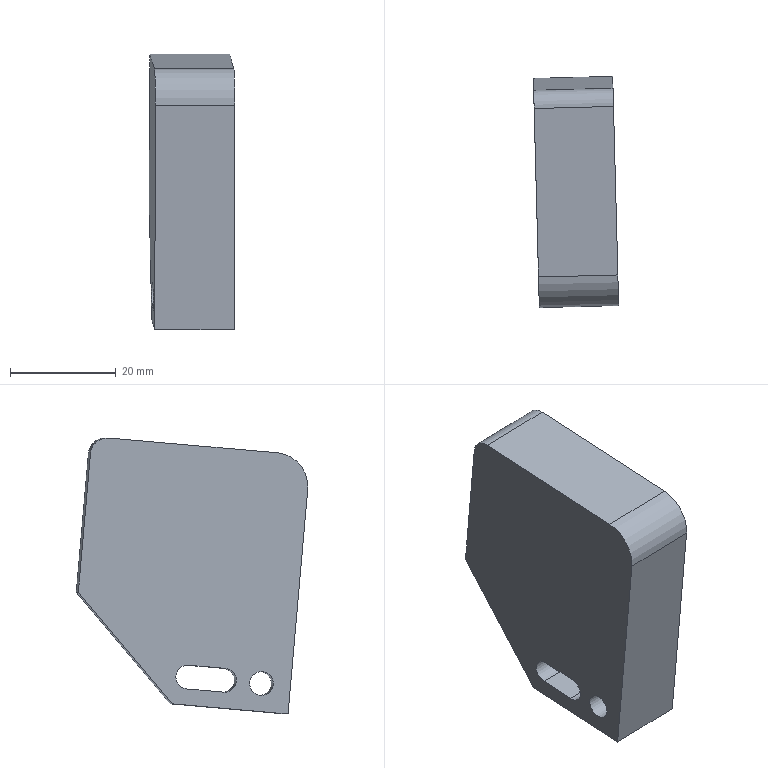Part | STEP file | 1_id1298_x_t | 1 solid | 14 faces | box 16.123 x 43.759 x 52.166 mm | volume 26539 mm3 | plane 9 | cylinder 5 | commonest cylinder face diameters 4.5 x3 6.35 x1 12.7 x1
STEP:
#1=CARTESIAN_POINT('',(0.,0.,0.));
#2=DIRECTION('',(0.,0.,1.));
#3=DIRECTION('',(1.,0.,0.));
#4=AXIS2_PLACEMENT_3D('',#1,#2,#3);
#5=CARTESIAN_POINT('',(981.211,308.005,19.618));
#6=VERTEX_POINT('',#5);
#7=CARTESIAN_POINT('',(966.216,307.615,19.618));
#8=VERTEX_POINT('',#7);
#9=CARTESIAN_POINT('',(981.211,308.005,19.618));
#10=DIRECTION('',(-0.9997,-0.02601,0.));
#11=VECTOR('',#10,1.);
#12=LINE('',#9,#11);
#13=CARTESIAN_POINT('',(981.114,311.721,-22.87));
#14=DIRECTION('',(0.02591,-0.9959,-0.08716));
#15=DIRECTION('',(0.05454,-0.08565,0.9948));
#16=AXIS2_PLACEMENT_3D('',#13,#14,#15);
#17=PLANE('',#16);
#18=CARTESIAN_POINT('',(42.592,2.23));
#19=DIRECTION('',(-0.0523,0.9986));
#20=VECTOR('',#19,1.);
#21=LINE('',#18,#20);
#22=(GEOMETRIC_REPRESENTATION_CONTEXT(2)PARAMETRIC_REPRESENTATION_CONTEXT()REPRESENTATION_CONTEXT('',''));
#23=DEFINITIONAL_REPRESENTATION('',(#21),#22);
#24=PCURVE('',#17,#23);
#25=CARTESIAN_POINT('',(981.046,314.328,20.171));
#26=DIRECTION('',(-0.9997,-0.02601,0.));
#27=DIRECTION('',(-0.01992,0.7658,-0.6428));
#28=AXIS2_PLACEMENT_3D('',#25,#26,#27);
#29=CYLINDRICAL_SURFACE('',#28,6.35);
#30=CARTESIAN_POINT('',(2.356,0.));
#31=DIRECTION('',(0.,1.));
#32=VECTOR('',#31,1.);
#33=LINE('',#30,#32);
#34=(GEOMETRIC_REPRESENTATION_CONTEXT(2)PARAMETRIC_REPRESENTATION_CONTEXT()REPRESENTATION_CONTEXT('',''));
#35=DEFINITIONAL_REPRESENTATION('',(#33),#34);
#36=PCURVE('',#29,#35);
#37=SURFACE_CURVE('',#12,(#24,#36),.PCURVE_S1.);
#38=EDGE_CURVE('',#6,#8,#37,.T.);
#39=ORIENTED_EDGE('',*,*,#38,.T.);
#40=CARTESIAN_POINT('',(966.119,311.331,-22.87));
#41=VERTEX_POINT('',#40);
#42=CARTESIAN_POINT('',(966.216,307.615,19.618));
#43=DIRECTION('',(-0.002266,0.08713,-0.9962));
#44=VECTOR('',#43,1.);
#45=LINE('',#42,#44);
#46=CARTESIAN_POINT('',(41.807,17.21));
#47=DIRECTION('',(-0.9986,-0.0523));
#48=VECTOR('',#47,1.);
#49=LINE('',#46,#48);
#50=(GEOMETRIC_REPRESENTATION_CONTEXT(2)PARAMETRIC_REPRESENTATION_CONTEXT()REPRESENTATION_CONTEXT('',''));
#51=DEFINITIONAL_REPRESENTATION('',(#49),#50);
#52=PCURVE('',#17,#51);
#53=CARTESIAN_POINT('',(966.23,307.061,25.943));
#54=DIRECTION('',(-0.9997,-0.02601,0.));
#55=DIRECTION('',(0.,0.,-1.));
#56=AXIS2_PLACEMENT_3D('',#53,#54,#55);
#57=PLANE('',#56);
#58=CARTESIAN_POINT('',(6.326,-0.5534));
#59=DIRECTION('',(0.9962,-0.08716));
#60=VECTOR('',#59,1.);
#61=LINE('',#58,#60);
#62=(GEOMETRIC_REPRESENTATION_CONTEXT(2)PARAMETRIC_REPRESENTATION_CONTEXT()REPRESENTATION_CONTEXT('',''));
#63=DEFINITIONAL_REPRESENTATION('',(#61),#62);
#64=PCURVE('',#57,#63);
#65=SURFACE_CURVE('',#45,(#52,#64),.PCURVE_S1.);
#66=EDGE_CURVE('',#8,#41,#65,.T.);
#67=ORIENTED_EDGE('',*,*,#66,.T.);
#68=CARTESIAN_POINT('',(981.114,311.721,-22.87));
#69=VERTEX_POINT('',#68);
#70=CARTESIAN_POINT('',(966.119,311.331,-22.87));
#71=DIRECTION('',(0.9997,0.02601,0.));
#72=VECTOR('',#71,1.);
#73=LINE('',#70,#72);
#74=CARTESIAN_POINT('',(-0.7845,14.979));
#75=DIRECTION('',(0.0523,-0.9986));
#76=VECTOR('',#75,1.);
#77=LINE('',#74,#76);
#78=(GEOMETRIC_REPRESENTATION_CONTEXT(2)PARAMETRIC_REPRESENTATION_CONTEXT()REPRESENTATION_CONTEXT('',''));
#79=DEFINITIONAL_REPRESENTATION('',(#77),#78);
#80=PCURVE('',#17,#79);
#81=CARTESIAN_POINT('',(980.544,333.629,-20.953));
#82=DIRECTION('',(-0.002266,0.08713,-0.9962));
#83=DIRECTION('',(0.8426,0.5366,0.04501));
#84=AXIS2_PLACEMENT_3D('',#81,#82,#83);
#85=PLANE('',#84);
#86=CARTESIAN_POINT('',(-24.207,11.091));
#87=DIRECTION('',(0.8563,0.5165));
#88=VECTOR('',#87,1.);
#89=LINE('',#86,#88);
#90=(GEOMETRIC_REPRESENTATION_CONTEXT(2)PARAMETRIC_REPRESENTATION_CONTEXT()REPRESENTATION_CONTEXT('',''));
#91=DEFINITIONAL_REPRESENTATION('',(#89),#90);
#92=PCURVE('',#85,#91);
#93=SURFACE_CURVE('',#73,(#80,#92),.PCURVE_S1.);
#94=EDGE_CURVE('',#41,#69,#93,.T.);
#95=ORIENTED_EDGE('',*,*,#94,.T.);
#96=CARTESIAN_POINT('',(981.211,308.005,19.618));
#97=DIRECTION('',(-0.002266,0.08713,-0.9962));
#98=VECTOR('',#97,1.);
#99=LINE('',#96,#98);
#100=CARTESIAN_POINT('',(42.592,2.23));
#101=DIRECTION('',(-0.9986,-0.0523));
#102=VECTOR('',#101,1.);
#103=LINE('',#100,#102);
#104=(GEOMETRIC_REPRESENTATION_CONTEXT(2)PARAMETRIC_REPRESENTATION_CONTEXT()REPRESENTATION_CONTEXT('',''));
#105=DEFINITIONAL_REPRESENTATION('',(#103),#104);
#106=PCURVE('',#17,#105);
#107=CARTESIAN_POINT('',(981.225,307.451,25.943));
#108=DIRECTION('',(-0.9997,-0.02601,0.));
#109=DIRECTION('',(0.,0.,-1.));
#110=AXIS2_PLACEMENT_3D('',#107,#108,#109);
#111=PLANE('',#110);
#112=CARTESIAN_POINT('',(6.326,-0.5534));
#113=DIRECTION('',(0.9962,-0.08716));
#114=VECTOR('',#113,1.);
#115=LINE('',#112,#114);
#116=(GEOMETRIC_REPRESENTATION_CONTEXT(2)PARAMETRIC_REPRESENTATION_CONTEXT()REPRESENTATION_CONTEXT('',''));
#117=DEFINITIONAL_REPRESENTATION('',(#115),#116);
#118=PCURVE('',#111,#117);
#119=SURFACE_CURVE('',#99,(#106,#118),.PCURVE_S1.);
#120=EDGE_CURVE('',#6,#69,#119,.T.);
#121=ORIENTED_EDGE('',*,*,#120,.F.);
#122=EDGE_LOOP('',(#39,#67,#95,#121));
#123=FACE_BOUND('',#122,.T.);
#124=ADVANCED_FACE('',(#123),#17,.T.);
#125=CARTESIAN_POINT('',(980.143,349.056,26.397));
#126=VERTEX_POINT('',#125);
#127=CARTESIAN_POINT('',(980.232,345.618,29.284));
#128=VERTEX_POINT('',#127);
#129=CARTESIAN_POINT('',(980.225,345.894,26.121));
#130=DIRECTION('',(0.9997,0.02601,0.));
#131=DIRECTION('',(-0.02591,0.9959,0.08716));
#132=AXIS2_PLACEMENT_3D('',#129,#130,#131);
#133=CIRCLE('',#132,3.175);
#134=CARTESIAN_POINT('',(-0.454,-41.619));
#135=CARTESIAN_POINT('',(-5.932,-41.14));
#136=CARTESIAN_POINT('',(-2.778,-36.635));
#137=CARTESIAN_POINT('',(0.3761,-32.13));
#138=CARTESIAN_POINT('',(2.7,-37.114));
#139=CARTESIAN_POINT('',(5.024,-42.098));
#140=CARTESIAN_POINT('',(-0.454,-41.619));
#141=(BOUNDED_CURVE()B_SPLINE_CURVE(2,(#134,#135,#136,#137,#138,#139,#140),.UNSPECIFIED.,.T.,.F.)B_SPLINE_CURVE_WITH_KNOTS((1,2,2,2,2,1),(-2.094,0.,2.094,4.189,6.283,8.378),.UNSPECIFIED.)CURVE()GEOMETRIC_REPRESENTATION_ITEM()RATIONAL_B_SPLINE_CURVE((1.,0.5,1.,0.5,1.,0.5,1.))REPRESENTATION_ITEM(''));
#142=(GEOMETRIC_REPRESENTATION_CONTEXT(2)PARAMETRIC_REPRESENTATION_CONTEXT()REPRESENTATION_CONTEXT('',''));
#143=DEFINITIONAL_REPRESENTATION('',(#141),#142);
#144=PCURVE('',#111,#143);
#145=CARTESIAN_POINT('',(980.225,345.894,26.121));
#146=DIRECTION('',(-0.9997,-0.02601,0.));
#147=DIRECTION('',(0.02591,-0.9959,-0.08716));
#148=AXIS2_PLACEMENT_3D('',#145,#146,#147);
#149=CYLINDRICAL_SURFACE('',#148,3.175);
#150=CARTESIAN_POINT('',(3.142,0.));
#151=DIRECTION('',(-1.,0.));
#152=VECTOR('',#151,1.);
#153=LINE('',#150,#152);
#154=(GEOMETRIC_REPRESENTATION_CONTEXT(2)PARAMETRIC_REPRESENTATION_CONTEXT()REPRESENTATION_CONTEXT('',''));
#155=DEFINITIONAL_REPRESENTATION('',(#153),#154);
#156=PCURVE('',#149,#155);
#157=SURFACE_CURVE('',#133,(#144,#156),.PCURVE_S1.);
#158=EDGE_CURVE('',#126,#128,#157,.T.);
#159=ORIENTED_EDGE('',*,*,#158,.T.);
#160=CARTESIAN_POINT('',(981.06,313.775,26.497));
#161=VERTEX_POINT('',#160);
#162=CARTESIAN_POINT('',(980.232,345.618,29.284));
#163=DIRECTION('',(0.02591,-0.9959,-0.08716));
#164=VECTOR('',#163,1.);
#165=LINE('',#162,#164);
#166=CARTESIAN_POINT('',(-3.34,-38.179));
#167=DIRECTION('',(0.08716,0.9962));
#168=VECTOR('',#167,1.);
#169=LINE('',#166,#168);
#170=(GEOMETRIC_REPRESENTATION_CONTEXT(2)PARAMETRIC_REPRESENTATION_CONTEXT()REPRESENTATION_CONTEXT('',''));
#171=DEFINITIONAL_REPRESENTATION('',(#169),#170);
#172=PCURVE('',#111,#171);
#173=CARTESIAN_POINT('',(981.225,307.451,25.943));
#174=DIRECTION('',(0.002266,-0.08713,0.9962));
#175=DIRECTION('',(-0.9997,-0.02601,0.));
#176=AXIS2_PLACEMENT_3D('',#173,#174,#175);
#177=PLANE('',#176);
#178=CARTESIAN_POINT('',(0.,-38.325));
#179=DIRECTION('',(0.,1.));
#180=VECTOR('',#179,1.);
#181=LINE('',#178,#180);
#182=(GEOMETRIC_REPRESENTATION_CONTEXT(2)PARAMETRIC_REPRESENTATION_CONTEXT()REPRESENTATION_CONTEXT('',''));
#183=DEFINITIONAL_REPRESENTATION('',(#181),#182);
#184=PCURVE('',#177,#183);
#185=SURFACE_CURVE('',#165,(#172,#184),.PCURVE_S1.);
#186=EDGE_CURVE('',#128,#161,#185,.T.);
#187=ORIENTED_EDGE('',*,*,#186,.T.);
#188=CARTESIAN_POINT('',(981.046,314.328,20.171));
#189=DIRECTION('',(0.9997,0.02601,0.));
#190=DIRECTION('',(0.01992,-0.7658,0.6428));
#191=AXIS2_PLACEMENT_3D('',#188,#189,#190);
#192=CIRCLE('',#191,6.35);
#193=CARTESIAN_POINT('',(1.691,-2.015));
#194=CARTESIAN_POINT('',(10.116,5.055));
#195=CARTESIAN_POINT('',(12.026,-5.777));
#196=CARTESIAN_POINT('',(13.936,-16.608));
#197=CARTESIAN_POINT('',(3.601,-12.846));
#198=CARTESIAN_POINT('',(-6.735,-9.085));
#199=CARTESIAN_POINT('',(1.691,-2.015));
#200=(BOUNDED_CURVE()B_SPLINE_CURVE(2,(#193,#194,#195,#196,#197,#198,#199),.UNSPECIFIED.,.T.,.F.)B_SPLINE_CURVE_WITH_KNOTS((1,2,2,2,2,1),(-2.094,0.,2.094,4.189,6.283,8.378),.UNSPECIFIED.)CURVE()GEOMETRIC_REPRESENTATION_ITEM()RATIONAL_B_SPLINE_CURVE((1.,0.5,1.,0.5,1.,0.5,1.))REPRESENTATION_ITEM(''));
#201=(GEOMETRIC_REPRESENTATION_CONTEXT(2)PARAMETRIC_REPRESENTATION_CONTEXT()REPRESENTATION_CONTEXT('',''));
#202=DEFINITIONAL_REPRESENTATION('',(#200),#201);
#203=PCURVE('',#111,#202);
#204=CARTESIAN_POINT('',(9.425,0.));
#205=DIRECTION('',(-1.,0.));
#206=VECTOR('',#205,1.);
#207=LINE('',#204,#206);
#208=(GEOMETRIC_REPRESENTATION_CONTEXT(2)PARAMETRIC_REPRESENTATION_CONTEXT()REPRESENTATION_CONTEXT('',''));
#209=DEFINITIONAL_REPRESENTATION('',(#207),#208);
#210=PCURVE('',#29,#209);
#211=SURFACE_CURVE('',#192,(#203,#210),.PCURVE_S1.);
#212=EDGE_CURVE('',#161,#6,#211,.T.);
#213=ORIENTED_EDGE('',*,*,#212,.T.);
#214=ORIENTED_EDGE('',*,*,#120,.T.);
#215=CARTESIAN_POINT('',(980.544,333.629,-20.953));
#216=VERTEX_POINT('',#215);
#217=CARTESIAN_POINT('',(981.114,311.721,-22.87));
#218=DIRECTION('',(-0.02591,0.9959,0.08716));
#219=VECTOR('',#218,1.);
#220=LINE('',#217,#219);
#221=CARTESIAN_POINT('',(48.814,-4.271));
#222=DIRECTION('',(-0.08716,-0.9962));
#223=VECTOR('',#222,1.);
#224=LINE('',#221,#223);
#225=(GEOMETRIC_REPRESENTATION_CONTEXT(2)PARAMETRIC_REPRESENTATION_CONTEXT()REPRESENTATION_CONTEXT('',''));
#226=DEFINITIONAL_REPRESENTATION('',(#224),#225);
#227=PCURVE('',#111,#226);
#228=CARTESIAN_POINT('',(-11.363,18.839));
#229=DIRECTION('',(0.5165,-0.8563));
#230=VECTOR('',#229,1.);
#231=LINE('',#228,#230);
#232=(GEOMETRIC_REPRESENTATION_CONTEXT(2)PARAMETRIC_REPRESENTATION_CONTEXT()REPRESENTATION_CONTEXT('',''));
#233=DEFINITIONAL_REPRESENTATION('',(#231),#232);
#234=PCURVE('',#85,#233);
#235=SURFACE_CURVE('',#220,(#227,#234),.PCURVE_S1.);
#236=EDGE_CURVE('',#69,#216,#235,.T.);
#237=ORIENTED_EDGE('',*,*,#236,.T.);
#238=CARTESIAN_POINT('',(980.083,351.35,0.1726));
#239=VERTEX_POINT('',#238);
#240=CARTESIAN_POINT('',(980.544,333.629,-20.953));
#241=DIRECTION('',(-0.01672,0.6426,0.766));
#242=VECTOR('',#241,1.);
#243=LINE('',#240,#242);
#244=CARTESIAN_POINT('',(46.896,-26.187));
#245=DIRECTION('',(-0.766,-0.6428));
#246=VECTOR('',#245,1.);
#247=LINE('',#244,#246);
#248=(GEOMETRIC_REPRESENTATION_CONTEXT(2)PARAMETRIC_REPRESENTATION_CONTEXT()REPRESENTATION_CONTEXT('',''));
#249=DEFINITIONAL_REPRESENTATION('',(#247),#248);
#250=PCURVE('',#111,#249);
#251=CARTESIAN_POINT('',(980.083,351.35,0.1726));
#252=DIRECTION('',(-0.01992,0.7658,-0.6428));
#253=DIRECTION('',(0.7189,0.4578,0.5231));
#254=AXIS2_PLACEMENT_3D('',#251,#252,#253);
#255=PLANE('',#254);
#256=CARTESIAN_POINT('',(-18.832,20.146));
#257=DIRECTION('',(0.6829,-0.7305));
#258=VECTOR('',#257,1.);
#259=LINE('',#256,#258);
#260=(GEOMETRIC_REPRESENTATION_CONTEXT(2)PARAMETRIC_REPRESENTATION_CONTEXT()REPRESENTATION_CONTEXT('',''));
#261=DEFINITIONAL_REPRESENTATION('',(#259),#260);
#262=PCURVE('',#255,#261);
#263=SURFACE_CURVE('',#243,(#250,#262),.PCURVE_S1.);
#264=EDGE_CURVE('',#216,#239,#263,.T.);
#265=ORIENTED_EDGE('',*,*,#264,.T.);
#266=CARTESIAN_POINT('',(980.083,351.35,0.1726));
#267=DIRECTION('',(0.002266,-0.08713,0.9962));
#268=VECTOR('',#267,1.);
#269=LINE('',#266,#268);
#270=CARTESIAN_POINT('',(25.771,-43.913));
#271=DIRECTION('',(-0.9962,0.08716));
#272=VECTOR('',#271,1.);
#273=LINE('',#270,#272);
#274=(GEOMETRIC_REPRESENTATION_CONTEXT(2)PARAMETRIC_REPRESENTATION_CONTEXT()REPRESENTATION_CONTEXT('',''));
#275=DEFINITIONAL_REPRESENTATION('',(#273),#274);
#276=PCURVE('',#111,#275);
#277=CARTESIAN_POINT('',(980.15,348.779,29.56));
#278=DIRECTION('',(-0.02591,0.9959,0.08716));
#279=DIRECTION('',(0.1413,0.08996,-0.9859));
#280=AXIS2_PLACEMENT_3D('',#277,#278,#279);
#281=PLANE('',#280);
#282=CARTESIAN_POINT('',(29.194,4.235));
#283=DIRECTION('',(-0.9896,-0.1435));
#284=VECTOR('',#283,1.);
#285=LINE('',#282,#284);
#286=(GEOMETRIC_REPRESENTATION_CONTEXT(2)PARAMETRIC_REPRESENTATION_CONTEXT()REPRESENTATION_CONTEXT('',''));
#287=DEFINITIONAL_REPRESENTATION('',(#285),#286);
#288=PCURVE('',#281,#287);
#289=SURFACE_CURVE('',#269,(#276,#288),.PCURVE_S1.);
#290=EDGE_CURVE('',#239,#126,#289,.T.);
#291=ORIENTED_EDGE('',*,*,#290,.T.);
#292=EDGE_LOOP('',(#159,#187,#213,#214,#237,#265,#291));
#293=FACE_BOUND('',#292,.T.);
#294=CARTESIAN_POINT('',(980.807,323.511,-14.259));
#295=VERTEX_POINT('',#294);
#296=CARTESIAN_POINT('',(980.626,330.482,-13.649));
#297=VERTEX_POINT('',#296);
#298=CARTESIAN_POINT('',(980.807,323.511,-14.259));
#299=DIRECTION('',(-0.02591,0.9959,0.08716));
#300=VECTOR('',#299,1.);
#301=LINE('',#298,#300);
#302=CARTESIAN_POINT('',(40.203,-16.065));
#303=DIRECTION('',(-0.08716,-0.9962));
#304=VECTOR('',#303,1.);
#305=LINE('',#302,#304);
#306=(GEOMETRIC_REPRESENTATION_CONTEXT(2)PARAMETRIC_REPRESENTATION_CONTEXT()REPRESENTATION_CONTEXT('',''));
#307=DEFINITIONAL_REPRESENTATION('',(#305),#306);
#308=PCURVE('',#111,#307);
#309=CARTESIAN_POINT('',(965.722,326.606,-13.954));
#310=DIRECTION('',(0.002266,-0.08713,0.9962));
#311=DIRECTION('',(-0.9997,-0.02601,0.));
#312=AXIS2_PLACEMENT_3D('',#309,#310,#311);
#313=PLANE('',#312);
#314=CARTESIAN_POINT('',(-15.,3.5));
#315=DIRECTION('',(0.,-1.));
#316=VECTOR('',#315,1.);
#317=LINE('',#314,#316);
#318=(GEOMETRIC_REPRESENTATION_CONTEXT(2)PARAMETRIC_REPRESENTATION_CONTEXT()REPRESENTATION_CONTEXT('',''));
#319=DEFINITIONAL_REPRESENTATION('',(#317),#318);
#320=PCURVE('',#313,#319);
#321=SURFACE_CURVE('',#301,(#308,#320),.PCURVE_S1.);
#322=EDGE_CURVE('',#295,#297,#321,.T.);
#323=ORIENTED_EDGE('',*,*,#322,.T.);
#324=CARTESIAN_POINT('',(980.616,330.874,-18.132));
#325=VERTEX_POINT('',#324);
#326=CARTESIAN_POINT('',(980.621,330.678,-15.891));
#327=DIRECTION('',(-0.9997,-0.02601,0.));
#328=DIRECTION('',(-0.02591,0.9959,0.08716));
#329=AXIS2_PLACEMENT_3D('',#326,#327,#328);
#330=CIRCLE('',#329,2.25);
#331=CARTESIAN_POINT('',(41.834,-23.235));
#332=DIRECTION('',(-0.08716,-0.9962));
#333=AXIS2_PLACEMENT_2D('',#331,#332);
#334=CIRCLE('',#333,2.25);
#335=(GEOMETRIC_REPRESENTATION_CONTEXT(2)PARAMETRIC_REPRESENTATION_CONTEXT()REPRESENTATION_CONTEXT('',''));
#336=DEFINITIONAL_REPRESENTATION('',(#334),#335);
#337=PCURVE('',#111,#336);
#338=CARTESIAN_POINT('',(965.626,330.288,-15.891));
#339=DIRECTION('',(-0.9997,-0.02601,0.));
#340=DIRECTION('',(0.02591,-0.9959,-0.08716));
#341=AXIS2_PLACEMENT_3D('',#338,#339,#340);
#342=CYLINDRICAL_SURFACE('',#341,2.25);
#343=CARTESIAN_POINT('',(-3.142,-15.));
#344=DIRECTION('',(1.,0.));
#345=VECTOR('',#344,1.);
#346=LINE('',#343,#345);
#347=(GEOMETRIC_REPRESENTATION_CONTEXT(2)PARAMETRIC_REPRESENTATION_CONTEXT()REPRESENTATION_CONTEXT('',''));
#348=DEFINITIONAL_REPRESENTATION('',(#346),#347);
#349=PCURVE('',#342,#348);
#350=SURFACE_CURVE('',#330,(#337,#349),.PCURVE_S1.);
#351=EDGE_CURVE('',#297,#325,#350,.T.);
#352=ORIENTED_EDGE('',*,*,#351,.T.);
#353=CARTESIAN_POINT('',(980.797,323.903,-18.742));
#354=VERTEX_POINT('',#353);
#355=CARTESIAN_POINT('',(980.797,323.903,-18.742));
#356=DIRECTION('',(-0.02591,0.9959,0.08716));
#357=VECTOR('',#356,1.);
#358=LINE('',#355,#357);
#359=CARTESIAN_POINT('',(44.686,-16.457));
#360=DIRECTION('',(-0.08716,-0.9962));
#361=VECTOR('',#360,1.);
#362=LINE('',#359,#361);
#363=(GEOMETRIC_REPRESENTATION_CONTEXT(2)PARAMETRIC_REPRESENTATION_CONTEXT()REPRESENTATION_CONTEXT('',''));
#364=DEFINITIONAL_REPRESENTATION('',(#362),#363);
#365=PCURVE('',#111,#364);
#366=CARTESIAN_POINT('',(965.711,326.998,-18.437));
#367=DIRECTION('',(-0.002266,0.08713,-0.9962));
#368=DIRECTION('',(0.8426,0.5366,0.04501));
#369=AXIS2_PLACEMENT_3D('',#366,#367,#368);
#370=PLANE('',#369);
#371=CARTESIAN_POINT('',(11.037,10.744));
#372=DIRECTION('',(0.5165,-0.8563));
#373=VECTOR('',#372,1.);
#374=LINE('',#371,#373);
#375=(GEOMETRIC_REPRESENTATION_CONTEXT(2)PARAMETRIC_REPRESENTATION_CONTEXT()REPRESENTATION_CONTEXT('',''));
#376=DEFINITIONAL_REPRESENTATION('',(#374),#375);
#377=PCURVE('',#370,#376);
#378=SURFACE_CURVE('',#358,(#365,#377),.PCURVE_S1.);
#379=EDGE_CURVE('',#354,#325,#378,.T.);
#380=ORIENTED_EDGE('',*,*,#379,.F.);
#381=CARTESIAN_POINT('',(980.802,323.707,-16.501));
#382=DIRECTION('',(-0.9997,-0.02601,0.));
#383=DIRECTION('',(0.02591,-0.9959,-0.08716));
#384=AXIS2_PLACEMENT_3D('',#381,#382,#383);
#385=CIRCLE('',#384,2.25);
#386=CARTESIAN_POINT('',(42.444,-16.261));
#387=DIRECTION('',(0.08716,0.9962));
#388=AXIS2_PLACEMENT_2D('',#386,#387);
#389=CIRCLE('',#388,2.25);
#390=(GEOMETRIC_REPRESENTATION_CONTEXT(2)PARAMETRIC_REPRESENTATION_CONTEXT()REPRESENTATION_CONTEXT('',''));
#391=DEFINITIONAL_REPRESENTATION('',(#389),#390);
#392=PCURVE('',#111,#391);
#393=CARTESIAN_POINT('',(965.807,323.317,-16.501));
#394=DIRECTION('',(-0.9997,-0.02601,0.));
#395=DIRECTION('',(-0.02591,0.9959,0.08716));
#396=AXIS2_PLACEMENT_3D('',#393,#394,#395);
#397=CYLINDRICAL_SURFACE('',#396,2.25);
#398=CARTESIAN_POINT('',(-3.142,-15.));
#399=DIRECTION('',(1.,0.));
#400=VECTOR('',#399,1.);
#401=LINE('',#398,#400);
#402=(GEOMETRIC_REPRESENTATION_CONTEXT(2)PARAMETRIC_REPRESENTATION_CONTEXT()REPRESENTATION_CONTEXT('',''));
#403=DEFINITIONAL_REPRESENTATION('',(#401),#402);
#404=PCURVE('',#397,#403);
#405=SURFACE_CURVE('',#385,(#392,#404),.PCURVE_S1.);
#406=EDGE_CURVE('',#354,#295,#405,.T.);
#407=ORIENTED_EDGE('',*,*,#406,.T.);
#408=EDGE_LOOP('',(#323,#352,#380,#407));
#409=FACE_BOUND('',#408,.T.);
#410=CARTESIAN_POINT('',(981.042,314.495,-17.307));
#411=VERTEX_POINT('',#410);
#412=CARTESIAN_POINT('',(980.983,316.736,-17.111));
#413=DIRECTION('',(-0.9997,-0.02601,0.));
#414=DIRECTION('',(0.02591,-0.9959,-0.08716));
#415=AXIS2_PLACEMENT_3D('',#412,#413,#414);
#416=CIRCLE('',#415,2.25);
#417=CARTESIAN_POINT('',(43.054,-9.288));
#418=DIRECTION('',(0.08716,0.9962));
#419=AXIS2_PLACEMENT_2D('',#417,#418);
#420=CIRCLE('',#419,2.25);
#421=(GEOMETRIC_REPRESENTATION_CONTEXT(2)PARAMETRIC_REPRESENTATION_CONTEXT()REPRESENTATION_CONTEXT('',''));
#422=DEFINITIONAL_REPRESENTATION('',(#420),#421);
#423=PCURVE('',#111,#422);
#424=CARTESIAN_POINT('',(965.988,316.346,-17.111));
#425=DIRECTION('',(0.9997,0.02601,0.));
#426=DIRECTION('',(0.02591,-0.9959,-0.08716));
#427=AXIS2_PLACEMENT_3D('',#424,#425,#426);
#428=CYLINDRICAL_SURFACE('',#427,2.25);
#429=CARTESIAN_POINT('',(6.283,15.));
#430=DIRECTION('',(-1.,0.));
#431=VECTOR('',#430,1.);
#432=LINE('',#429,#431);
#433=(GEOMETRIC_REPRESENTATION_CONTEXT(2)PARAMETRIC_REPRESENTATION_CONTEXT()REPRESENTATION_CONTEXT('',''));
#434=DEFINITIONAL_REPRESENTATION('',(#432),#433);
#435=PCURVE('',#428,#434);
#436=SURFACE_CURVE('',#416,(#423,#435),.PCURVE_S1.);
#437=EDGE_CURVE('',#411,#411,#436,.T.);
#438=ORIENTED_EDGE('',*,*,#437,.T.);
#439=EDGE_LOOP('',(#438));
#440=FACE_BOUND('',#439,.T.);
#441=ADVANCED_FACE('',(#293,#409,#440),#111,.F.);
#442=CARTESIAN_POINT('',(965.148,348.666,26.397));
#443=VERTEX_POINT('',#442);
#444=CARTESIAN_POINT('',(965.148,348.666,26.397));
#445=DIRECTION('',(0.9997,0.02601,0.));
#446=VECTOR('',#445,1.);
#447=LINE('',#444,#446);
#448=CARTESIAN_POINT('',(0.9889,15.3));
#449=DIRECTION('',(0.1435,-0.9896));
#450=VECTOR('',#449,1.);
#451=LINE('',#448,#450);
#452=(GEOMETRIC_REPRESENTATION_CONTEXT(2)PARAMETRIC_REPRESENTATION_CONTEXT()REPRESENTATION_CONTEXT('',''));
#453=DEFINITIONAL_REPRESENTATION('',(#451),#452);
#454=PCURVE('',#281,#453);
#455=CARTESIAN_POINT('',(3.142,15.));
#456=DIRECTION('',(0.,-1.));
#457=VECTOR('',#456,1.);
#458=LINE('',#455,#457);
#459=(GEOMETRIC_REPRESENTATION_CONTEXT(2)PARAMETRIC_REPRESENTATION_CONTEXT()REPRESENTATION_CONTEXT('',''));
#460=DEFINITIONAL_REPRESENTATION('',(#458),#459);
#461=PCURVE('',#149,#460);
#462=SURFACE_CURVE('',#447,(#454,#461),.PCURVE_S1.);
#463=EDGE_CURVE('',#443,#126,#462,.T.);
#464=ORIENTED_EDGE('',*,*,#463,.T.);
#465=ORIENTED_EDGE('',*,*,#290,.F.);
#466=CARTESIAN_POINT('',(965.088,350.96,0.1726));
#467=VERTEX_POINT('',#466);
#468=CARTESIAN_POINT('',(965.088,350.96,0.1726));
#469=DIRECTION('',(0.9997,0.02601,0.));
#470=VECTOR('',#469,1.);
#471=LINE('',#468,#470);
#472=CARTESIAN_POINT('',(27.041,19.079));
#473=DIRECTION('',(0.1435,-0.9896));
#474=VECTOR('',#473,1.);
#475=LINE('',#472,#474);
#476=(GEOMETRIC_REPRESENTATION_CONTEXT(2)PARAMETRIC_REPRESENTATION_CONTEXT()REPRESENTATION_CONTEXT('',''));
#477=DEFINITIONAL_REPRESENTATION('',(#475),#476);
#478=PCURVE('',#281,#477);
#479=CARTESIAN_POINT('',(-10.958,-10.243));
#480=DIRECTION('',(0.7305,0.6829));
#481=VECTOR('',#480,1.);
#482=LINE('',#479,#481);
#483=(GEOMETRIC_REPRESENTATION_CONTEXT(2)PARAMETRIC_REPRESENTATION_CONTEXT()REPRESENTATION_CONTEXT('',''));
#484=DEFINITIONAL_REPRESENTATION('',(#482),#483);
#485=PCURVE('',#255,#484);
#486=SURFACE_CURVE('',#471,(#478,#485),.PCURVE_S1.);
#487=EDGE_CURVE('',#467,#239,#486,.T.);
#488=ORIENTED_EDGE('',*,*,#487,.F.);
#489=CARTESIAN_POINT('',(965.088,350.96,0.1726));
#490=DIRECTION('',(0.002266,-0.08713,0.9962));
#491=VECTOR('',#490,1.);
#492=LINE('',#489,#491);
#493=CARTESIAN_POINT('',(27.041,19.079));
#494=DIRECTION('',(-0.9896,-0.1435));
#495=VECTOR('',#494,1.);
#496=LINE('',#493,#495);
#497=(GEOMETRIC_REPRESENTATION_CONTEXT(2)PARAMETRIC_REPRESENTATION_CONTEXT()REPRESENTATION_CONTEXT('',''));
#498=DEFINITIONAL_REPRESENTATION('',(#496),#497);
#499=PCURVE('',#281,#498);
#500=CARTESIAN_POINT('',(25.771,-43.913));
#501=DIRECTION('',(-0.9962,0.08716));
#502=VECTOR('',#501,1.);
#503=LINE('',#500,#502);
#504=(GEOMETRIC_REPRESENTATION_CONTEXT(2)PARAMETRIC_REPRESENTATION_CONTEXT()REPRESENTATION_CONTEXT('',''));
#505=DEFINITIONAL_REPRESENTATION('',(#503),#504);
#506=PCURVE('',#57,#505);
#507=SURFACE_CURVE('',#492,(#499,#506),.PCURVE_S1.);
#508=EDGE_CURVE('',#467,#443,#507,.T.);
#509=ORIENTED_EDGE('',*,*,#508,.T.);
#510=EDGE_LOOP('',(#464,#465,#488,#509));
#511=FACE_BOUND('',#510,.T.);
#512=ADVANCED_FACE('',(#511),#281,.T.);
#513=CARTESIAN_POINT('',(965.237,345.228,29.284));
#514=VERTEX_POINT('',#513);
#515=CARTESIAN_POINT('',(965.23,345.504,26.121));
#516=DIRECTION('',(-0.9997,-0.02601,0.));
#517=DIRECTION('',(0.002266,-0.08713,0.9962));
#518=AXIS2_PLACEMENT_3D('',#515,#516,#517);
#519=CIRCLE('',#518,3.175);
#520=CARTESIAN_POINT('',(-0.1773,-38.456));
#521=DIRECTION('',(-0.9962,0.08716));
#522=AXIS2_PLACEMENT_2D('',#520,#521);
#523=CIRCLE('',#522,3.175);
#524=(GEOMETRIC_REPRESENTATION_CONTEXT(2)PARAMETRIC_REPRESENTATION_CONTEXT()REPRESENTATION_CONTEXT('',''));
#525=DEFINITIONAL_REPRESENTATION('',(#523),#524);
#526=PCURVE('',#57,#525);
#527=CARTESIAN_POINT('',(1.571,15.));
#528=DIRECTION('',(1.,0.));
#529=VECTOR('',#528,1.);
#530=LINE('',#527,#529);
#531=(GEOMETRIC_REPRESENTATION_CONTEXT(2)PARAMETRIC_REPRESENTATION_CONTEXT()REPRESENTATION_CONTEXT('',''));
#532=DEFINITIONAL_REPRESENTATION('',(#530),#531);
#533=PCURVE('',#149,#532);
#534=SURFACE_CURVE('',#519,(#526,#533),.PCURVE_S1.);
#535=EDGE_CURVE('',#514,#443,#534,.T.);
#536=ORIENTED_EDGE('',*,*,#535,.T.);
#537=ORIENTED_EDGE('',*,*,#508,.F.);
#538=CARTESIAN_POINT('',(965.549,333.239,-20.953));
#539=VERTEX_POINT('',#538);
#540=CARTESIAN_POINT('',(965.549,333.239,-20.953));
#541=DIRECTION('',(-0.01672,0.6426,0.766));
#542=VECTOR('',#541,1.);
#543=LINE('',#540,#542);
#544=CARTESIAN_POINT('',(46.896,-26.187));
#545=DIRECTION('',(-0.766,-0.6428));
#546=VECTOR('',#545,1.);
#547=LINE('',#544,#546);
#548=(GEOMETRIC_REPRESENTATION_CONTEXT(2)PARAMETRIC_REPRESENTATION_CONTEXT()REPRESENTATION_CONTEXT('',''));
#549=DEFINITIONAL_REPRESENTATION('',(#547),#548);
#550=PCURVE('',#57,#549);
#551=CARTESIAN_POINT('',(-29.79,9.903));
#552=DIRECTION('',(0.6829,-0.7305));
#553=VECTOR('',#552,1.);
#554=LINE('',#551,#553);
#555=(GEOMETRIC_REPRESENTATION_CONTEXT(2)PARAMETRIC_REPRESENTATION_CONTEXT()REPRESENTATION_CONTEXT('',''));
#556=DEFINITIONAL_REPRESENTATION('',(#554),#555);
#557=PCURVE('',#255,#556);
#558=SURFACE_CURVE('',#543,(#550,#557),.PCURVE_S1.);
#559=EDGE_CURVE('',#539,#467,#558,.T.);
#560=ORIENTED_EDGE('',*,*,#559,.F.);
#561=CARTESIAN_POINT('',(966.119,311.331,-22.87));
#562=DIRECTION('',(-0.02591,0.9959,0.08716));
#563=VECTOR('',#562,1.);
#564=LINE('',#561,#563);
#565=CARTESIAN_POINT('',(48.814,-4.271));
#566=DIRECTION('',(-0.08716,-0.9962));
#567=VECTOR('',#566,1.);
#568=LINE('',#565,#567);
#569=(GEOMETRIC_REPRESENTATION_CONTEXT(2)PARAMETRIC_REPRESENTATION_CONTEXT()REPRESENTATION_CONTEXT('',''));
#570=DEFINITIONAL_REPRESENTATION('',(#568),#569);
#571=PCURVE('',#57,#570);
#572=CARTESIAN_POINT('',(-24.207,11.091));
#573=DIRECTION('',(0.5165,-0.8563));
#574=VECTOR('',#573,1.);
#575=LINE('',#572,#574);
#576=(GEOMETRIC_REPRESENTATION_CONTEXT(2)PARAMETRIC_REPRESENTATION_CONTEXT()REPRESENTATION_CONTEXT('',''));
#577=DEFINITIONAL_REPRESENTATION('',(#575),#576);
#578=PCURVE('',#85,#577);
#579=SURFACE_CURVE('',#564,(#571,#578),.PCURVE_S1.);
#580=EDGE_CURVE('',#41,#539,#579,.T.);
#581=ORIENTED_EDGE('',*,*,#580,.F.);
#582=ORIENTED_EDGE('',*,*,#66,.F.);
#583=CARTESIAN_POINT('',(966.066,313.385,26.497));
#584=VERTEX_POINT('',#583);
#585=CARTESIAN_POINT('',(966.051,313.938,20.171));
#586=DIRECTION('',(-0.9997,-0.02601,0.));
#587=DIRECTION('',(0.01992,-0.7658,0.6428));
#588=AXIS2_PLACEMENT_3D('',#585,#586,#587);
#589=CIRCLE('',#588,6.35);
#590=CARTESIAN_POINT('',(5.772,-6.879));
#591=DIRECTION('',(-0.6428,0.766));
#592=AXIS2_PLACEMENT_2D('',#590,#591);
#593=CIRCLE('',#592,6.35);
#594=(GEOMETRIC_REPRESENTATION_CONTEXT(2)PARAMETRIC_REPRESENTATION_CONTEXT()REPRESENTATION_CONTEXT('',''));
#595=DEFINITIONAL_REPRESENTATION('',(#593),#594);
#596=PCURVE('',#57,#595);
#597=CARTESIAN_POINT('',(-3.142,15.));
#598=DIRECTION('',(1.,0.));
#599=VECTOR('',#598,1.);
#600=LINE('',#597,#599);
#601=(GEOMETRIC_REPRESENTATION_CONTEXT(2)PARAMETRIC_REPRESENTATION_CONTEXT()REPRESENTATION_CONTEXT('',''));
#602=DEFINITIONAL_REPRESENTATION('',(#600),#601);
#603=PCURVE('',#29,#602);
#604=SURFACE_CURVE('',#589,(#596,#603),.PCURVE_S1.);
#605=EDGE_CURVE('',#8,#584,#604,.T.);
#606=ORIENTED_EDGE('',*,*,#605,.T.);
#607=CARTESIAN_POINT('',(966.066,313.385,26.497));
#608=DIRECTION('',(-0.02591,0.9959,0.08716));
#609=VECTOR('',#608,1.);
#610=LINE('',#607,#609);
#611=CARTESIAN_POINT('',(-0.5534,-6.326));
#612=DIRECTION('',(-0.08716,-0.9962));
#613=VECTOR('',#612,1.);
#614=LINE('',#611,#613);
#615=(GEOMETRIC_REPRESENTATION_CONTEXT(2)PARAMETRIC_REPRESENTATION_CONTEXT()REPRESENTATION_CONTEXT('',''));
#616=DEFINITIONAL_REPRESENTATION('',(#614),#615);
#617=PCURVE('',#57,#616);
#618=CARTESIAN_POINT('',(15.,-6.35));
#619=DIRECTION('',(0.,-1.));
#620=VECTOR('',#619,1.);
#621=LINE('',#618,#620);
#622=(GEOMETRIC_REPRESENTATION_CONTEXT(2)PARAMETRIC_REPRESENTATION_CONTEXT()REPRESENTATION_CONTEXT('',''));
#623=DEFINITIONAL_REPRESENTATION('',(#621),#622);
#624=PCURVE('',#177,#623);
#625=SURFACE_CURVE('',#610,(#617,#624),.PCURVE_S1.);
#626=EDGE_CURVE('',#584,#514,#625,.T.);
#627=ORIENTED_EDGE('',*,*,#626,.T.);
#628=EDGE_LOOP('',(#536,#537,#560,#581,#582,#606,#627));
#629=FACE_BOUND('',#628,.T.);
#630=CARTESIAN_POINT('',(965.621,330.484,-18.132));
#631=VERTEX_POINT('',#630);
#632=CARTESIAN_POINT('',(965.802,323.513,-18.742));
#633=VERTEX_POINT('',#632);
#634=CARTESIAN_POINT('',(965.621,330.484,-18.132));
#635=DIRECTION('',(0.02591,-0.9959,-0.08716));
#636=VECTOR('',#635,1.);
#637=LINE('',#634,#636);
#638=CARTESIAN_POINT('',(44.076,-23.431));
#639=DIRECTION('',(0.08716,0.9962));
#640=VECTOR('',#639,1.);
#641=LINE('',#638,#640);
#642=(GEOMETRIC_REPRESENTATION_CONTEXT(2)PARAMETRIC_REPRESENTATION_CONTEXT()REPRESENTATION_CONTEXT('',''));
#643=DEFINITIONAL_REPRESENTATION('',(#641),#642);
#644=PCURVE('',#57,#643);
#645=CARTESIAN_POINT('',(1.808,-2.997));
#646=DIRECTION('',(-0.5165,0.8563));
#647=VECTOR('',#646,1.);
#648=LINE('',#645,#647);
#649=(GEOMETRIC_REPRESENTATION_CONTEXT(2)PARAMETRIC_REPRESENTATION_CONTEXT()REPRESENTATION_CONTEXT('',''));
#650=DEFINITIONAL_REPRESENTATION('',(#648),#649);
#651=PCURVE('',#370,#650);
#652=SURFACE_CURVE('',#637,(#644,#651),.PCURVE_S1.);
#653=EDGE_CURVE('',#631,#633,#652,.T.);
#654=ORIENTED_EDGE('',*,*,#653,.F.);
#655=CARTESIAN_POINT('',(965.631,330.092,-13.649));
#656=VERTEX_POINT('',#655);
#657=CARTESIAN_POINT('',(965.626,330.288,-15.891));
#658=DIRECTION('',(0.9997,0.02601,0.));
#659=DIRECTION('',(-0.02591,0.9959,0.08716));
#660=AXIS2_PLACEMENT_3D('',#657,#658,#659);
#661=CIRCLE('',#660,2.25);
#662=CARTESIAN_POINT('',(41.638,-25.476));
#663=CARTESIAN_POINT('',(37.756,-25.136));
#664=CARTESIAN_POINT('',(39.991,-21.944));
#665=CARTESIAN_POINT('',(42.226,-18.752));
#666=CARTESIAN_POINT('',(43.873,-22.284));
#667=CARTESIAN_POINT('',(45.52,-25.816));
#668=CARTESIAN_POINT('',(41.638,-25.476));
#669=(BOUNDED_CURVE()B_SPLINE_CURVE(2,(#662,#663,#664,#665,#666,#667,#668),.UNSPECIFIED.,.T.,.F.)B_SPLINE_CURVE_WITH_KNOTS((1,2,2,2,2,1),(-2.094,0.,2.094,4.189,6.283,8.378),.UNSPECIFIED.)CURVE()GEOMETRIC_REPRESENTATION_ITEM()RATIONAL_B_SPLINE_CURVE((1.,0.5,1.,0.5,1.,0.5,1.))REPRESENTATION_ITEM(''));
#670=(GEOMETRIC_REPRESENTATION_CONTEXT(2)PARAMETRIC_REPRESENTATION_CONTEXT()REPRESENTATION_CONTEXT('',''));
#671=DEFINITIONAL_REPRESENTATION('',(#669),#670);
#672=PCURVE('',#57,#671);
#673=CARTESIAN_POINT('',(9.425,0.));
#674=DIRECTION('',(-1.,0.));
#675=VECTOR('',#674,1.);
#676=LINE('',#673,#675);
#677=(GEOMETRIC_REPRESENTATION_CONTEXT(2)PARAMETRIC_REPRESENTATION_CONTEXT()REPRESENTATION_CONTEXT('',''));
#678=DEFINITIONAL_REPRESENTATION('',(#676),#677);
#679=PCURVE('',#342,#678);
#680=SURFACE_CURVE('',#661,(#672,#679),.PCURVE_S1.);
#681=EDGE_CURVE('',#631,#656,#680,.T.);
#682=ORIENTED_EDGE('',*,*,#681,.T.);
#683=CARTESIAN_POINT('',(965.812,323.121,-14.259));
#684=VERTEX_POINT('',#683);
#685=CARTESIAN_POINT('',(965.631,330.092,-13.649));
#686=DIRECTION('',(0.02591,-0.9959,-0.08716));
#687=VECTOR('',#686,1.);
#688=LINE('',#685,#687);
#689=CARTESIAN_POINT('',(39.593,-23.038));
#690=DIRECTION('',(0.08716,0.9962));
#691=VECTOR('',#690,1.);
#692=LINE('',#689,#691);
#693=(GEOMETRIC_REPRESENTATION_CONTEXT(2)PARAMETRIC_REPRESENTATION_CONTEXT()REPRESENTATION_CONTEXT('',''));
#694=DEFINITIONAL_REPRESENTATION('',(#692),#693);
#695=PCURVE('',#57,#694);
#696=CARTESIAN_POINT('',(0.,-3.5));
#697=DIRECTION('',(0.,1.));
#698=VECTOR('',#697,1.);
#699=LINE('',#696,#698);
#700=(GEOMETRIC_REPRESENTATION_CONTEXT(2)PARAMETRIC_REPRESENTATION_CONTEXT()REPRESENTATION_CONTEXT('',''));
#701=DEFINITIONAL_REPRESENTATION('',(#699),#700);
#702=PCURVE('',#313,#701);
#703=SURFACE_CURVE('',#688,(#695,#702),.PCURVE_S1.);
#704=EDGE_CURVE('',#656,#684,#703,.T.);
#705=ORIENTED_EDGE('',*,*,#704,.T.);
#706=CARTESIAN_POINT('',(965.807,323.317,-16.501));
#707=DIRECTION('',(0.9997,0.02601,0.));
#708=DIRECTION('',(0.02591,-0.9959,-0.08716));
#709=AXIS2_PLACEMENT_3D('',#706,#707,#708);
#710=CIRCLE('',#709,2.25);
#711=CARTESIAN_POINT('',(42.64,-14.02));
#712=CARTESIAN_POINT('',(46.523,-14.359));
#713=CARTESIAN_POINT('',(44.287,-17.552));
#714=CARTESIAN_POINT('',(42.052,-20.744));
#715=CARTESIAN_POINT('',(40.405,-17.212));
#716=CARTESIAN_POINT('',(38.758,-13.68));
#717=CARTESIAN_POINT('',(42.64,-14.02));
#718=(BOUNDED_CURVE()B_SPLINE_CURVE(2,(#711,#712,#713,#714,#715,#716,#717),.UNSPECIFIED.,.T.,.F.)B_SPLINE_CURVE_WITH_KNOTS((1,2,2,2,2,1),(-2.094,0.,2.094,4.189,6.283,8.378),.UNSPECIFIED.)CURVE()GEOMETRIC_REPRESENTATION_ITEM()RATIONAL_B_SPLINE_CURVE((1.,0.5,1.,0.5,1.,0.5,1.))REPRESENTATION_ITEM(''));
#719=(GEOMETRIC_REPRESENTATION_CONTEXT(2)PARAMETRIC_REPRESENTATION_CONTEXT()REPRESENTATION_CONTEXT('',''));
#720=DEFINITIONAL_REPRESENTATION('',(#718),#719);
#721=PCURVE('',#57,#720);
#722=CARTESIAN_POINT('',(9.425,0.));
#723=DIRECTION('',(-1.,0.));
#724=VECTOR('',#723,1.);
#725=LINE('',#722,#724);
#726=(GEOMETRIC_REPRESENTATION_CONTEXT(2)PARAMETRIC_REPRESENTATION_CONTEXT()REPRESENTATION_CONTEXT('',''));
#727=DEFINITIONAL_REPRESENTATION('',(#725),#726);
#728=PCURVE('',#397,#727);
#729=SURFACE_CURVE('',#710,(#721,#728),.PCURVE_S1.);
#730=EDGE_CURVE('',#684,#633,#729,.T.);
#731=ORIENTED_EDGE('',*,*,#730,.T.);
#732=EDGE_LOOP('',(#654,#682,#705,#731));
#733=FACE_BOUND('',#732,.T.);
#734=CARTESIAN_POINT('',(966.047,314.105,-17.307));
#735=VERTEX_POINT('',#734);
#736=CARTESIAN_POINT('',(965.988,316.346,-17.111));
#737=DIRECTION('',(0.9997,0.02601,0.));
#738=DIRECTION('',(0.02591,-0.9959,-0.08716));
#739=AXIS2_PLACEMENT_3D('',#736,#737,#738);
#740=CIRCLE('',#739,2.25);
#741=CARTESIAN_POINT('',(43.25,-7.046));
#742=CARTESIAN_POINT('',(47.133,-7.386));
#743=CARTESIAN_POINT('',(44.897,-10.578));
#744=CARTESIAN_POINT('',(42.662,-13.771));
#745=CARTESIAN_POINT('',(41.015,-10.239));
#746=CARTESIAN_POINT('',(39.368,-6.707));
#747=CARTESIAN_POINT('',(43.25,-7.046));
#748=(BOUNDED_CURVE()B_SPLINE_CURVE(2,(#741,#742,#743,#744,#745,#746,#747),.UNSPECIFIED.,.T.,.F.)B_SPLINE_CURVE_WITH_KNOTS((1,2,2,2,2,1),(-2.094,0.,2.094,4.189,6.283,8.378),.UNSPECIFIED.)CURVE()GEOMETRIC_REPRESENTATION_ITEM()RATIONAL_B_SPLINE_CURVE((1.,0.5,1.,0.5,1.,0.5,1.))REPRESENTATION_ITEM(''));
#749=(GEOMETRIC_REPRESENTATION_CONTEXT(2)PARAMETRIC_REPRESENTATION_CONTEXT()REPRESENTATION_CONTEXT('',''));
#750=DEFINITIONAL_REPRESENTATION('',(#748),#749);
#751=PCURVE('',#57,#750);
#752=CARTESIAN_POINT('',(0.,0.));
#753=DIRECTION('',(1.,0.));
#754=VECTOR('',#753,1.);
#755=LINE('',#752,#754);
#756=(GEOMETRIC_REPRESENTATION_CONTEXT(2)PARAMETRIC_REPRESENTATION_CONTEXT()REPRESENTATION_CONTEXT('',''));
#757=DEFINITIONAL_REPRESENTATION('',(#755),#756);
#758=PCURVE('',#428,#757);
#759=SURFACE_CURVE('',#740,(#751,#758),.PCURVE_S1.);
#760=EDGE_CURVE('',#735,#735,#759,.T.);
#761=ORIENTED_EDGE('',*,*,#760,.T.);
#762=EDGE_LOOP('',(#761));
#763=FACE_BOUND('',#762,.T.);
#764=ADVANCED_FACE('',(#629,#733,#763),#57,.T.);
#765=CARTESIAN_POINT('',(965.237,345.228,29.284));
#766=DIRECTION('',(0.9997,0.02601,0.));
#767=VECTOR('',#766,1.);
#768=LINE('',#765,#767);
#769=CARTESIAN_POINT('',(15.,-38.325));
#770=DIRECTION('',(-1.,0.));
#771=VECTOR('',#770,1.);
#772=LINE('',#769,#771);
#773=(GEOMETRIC_REPRESENTATION_CONTEXT(2)PARAMETRIC_REPRESENTATION_CONTEXT()REPRESENTATION_CONTEXT('',''));
#774=DEFINITIONAL_REPRESENTATION('',(#772),#773);
#775=PCURVE('',#177,#774);
#776=CARTESIAN_POINT('',(1.571,15.));
#777=DIRECTION('',(0.,-1.));
#778=VECTOR('',#777,1.);
#779=LINE('',#776,#778);
#780=(GEOMETRIC_REPRESENTATION_CONTEXT(2)PARAMETRIC_REPRESENTATION_CONTEXT()REPRESENTATION_CONTEXT('',''));
#781=DEFINITIONAL_REPRESENTATION('',(#779),#780);
#782=PCURVE('',#149,#781);
#783=SURFACE_CURVE('',#768,(#775,#782),.PCURVE_S1.);
#784=EDGE_CURVE('',#514,#128,#783,.T.);
#785=ORIENTED_EDGE('',*,*,#784,.F.);
#786=ORIENTED_EDGE('',*,*,#626,.F.);
#787=CARTESIAN_POINT('',(981.06,313.775,26.497));
#788=DIRECTION('',(-0.9997,-0.02601,0.));
#789=VECTOR('',#788,1.);
#790=LINE('',#787,#789);
#791=CARTESIAN_POINT('',(0.,-6.35));
#792=DIRECTION('',(1.,0.));
#793=VECTOR('',#792,1.);
#794=LINE('',#791,#793);
#795=(GEOMETRIC_REPRESENTATION_CONTEXT(2)PARAMETRIC_REPRESENTATION_CONTEXT()REPRESENTATION_CONTEXT('',''));
#796=DEFINITIONAL_REPRESENTATION('',(#794),#795);
#797=PCURVE('',#177,#796);
#798=CARTESIAN_POINT('',(3.927,0.));
#799=DIRECTION('',(0.,1.));
#800=VECTOR('',#799,1.);
#801=LINE('',#798,#800);
#802=(GEOMETRIC_REPRESENTATION_CONTEXT(2)PARAMETRIC_REPRESENTATION_CONTEXT()REPRESENTATION_CONTEXT('',''));
#803=DEFINITIONAL_REPRESENTATION('',(#801),#802);
#804=PCURVE('',#29,#803);
#805=SURFACE_CURVE('',#790,(#797,#804),.PCURVE_S1.);
#806=EDGE_CURVE('',#161,#584,#805,.T.);
#807=ORIENTED_EDGE('',*,*,#806,.F.);
#808=ORIENTED_EDGE('',*,*,#186,.F.);
#809=EDGE_LOOP('',(#785,#786,#807,#808));
#810=FACE_BOUND('',#809,.T.);
#811=ADVANCED_FACE('',(#810),#177,.T.);
#812=ORIENTED_EDGE('',*,*,#212,.F.);
#813=ORIENTED_EDGE('',*,*,#806,.T.);
#814=ORIENTED_EDGE('',*,*,#605,.F.);
#815=ORIENTED_EDGE('',*,*,#38,.F.);
#816=EDGE_LOOP('',(#812,#813,#814,#815));
#817=FACE_BOUND('',#816,.T.);
#818=ADVANCED_FACE('',(#817),#29,.T.);
#819=ORIENTED_EDGE('',*,*,#463,.F.);
#820=ORIENTED_EDGE('',*,*,#535,.F.);
#821=ORIENTED_EDGE('',*,*,#784,.T.);
#822=ORIENTED_EDGE('',*,*,#158,.F.);
#823=EDGE_LOOP('',(#819,#820,#821,#822));
#824=FACE_BOUND('',#823,.T.);
#825=ADVANCED_FACE('',(#824),#149,.T.);
#826=CARTESIAN_POINT('',(965.549,333.239,-20.953));
#827=DIRECTION('',(0.9997,0.02601,0.));
#828=VECTOR('',#827,1.);
#829=LINE('',#826,#828);
#830=CARTESIAN_POINT('',(-12.844,-7.747));
#831=DIRECTION('',(0.8563,0.5165));
#832=VECTOR('',#831,1.);
#833=LINE('',#830,#832);
#834=(GEOMETRIC_REPRESENTATION_CONTEXT(2)PARAMETRIC_REPRESENTATION_CONTEXT()REPRESENTATION_CONTEXT('',''));
#835=DEFINITIONAL_REPRESENTATION('',(#833),#834);
#836=PCURVE('',#85,#835);
#837=CARTESIAN_POINT('',(-29.79,9.903));
#838=DIRECTION('',(0.7305,0.6829));
#839=VECTOR('',#838,1.);
#840=LINE('',#837,#839);
#841=(GEOMETRIC_REPRESENTATION_CONTEXT(2)PARAMETRIC_REPRESENTATION_CONTEXT()REPRESENTATION_CONTEXT('',''));
#842=DEFINITIONAL_REPRESENTATION('',(#840),#841);
#843=PCURVE('',#255,#842);
#844=SURFACE_CURVE('',#829,(#836,#843),.PCURVE_S1.);
#845=EDGE_CURVE('',#539,#216,#844,.T.);
#846=ORIENTED_EDGE('',*,*,#845,.T.);
#847=ORIENTED_EDGE('',*,*,#236,.F.);
#848=ORIENTED_EDGE('',*,*,#94,.F.);
#849=ORIENTED_EDGE('',*,*,#580,.T.);
#850=EDGE_LOOP('',(#846,#847,#848,#849));
#851=FACE_BOUND('',#850,.T.);
#852=ADVANCED_FACE('',(#851),#85,.T.);
#853=ORIENTED_EDGE('',*,*,#487,.T.);
#854=ORIENTED_EDGE('',*,*,#264,.F.);
#855=ORIENTED_EDGE('',*,*,#845,.F.);
#856=ORIENTED_EDGE('',*,*,#559,.T.);
#857=EDGE_LOOP('',(#853,#854,#855,#856));
#858=FACE_BOUND('',#857,.T.);
#859=ADVANCED_FACE('',(#858),#255,.T.);
#860=CARTESIAN_POINT('',(965.802,323.513,-18.742));
#861=DIRECTION('',(0.9997,0.02601,0.));
#862=VECTOR('',#861,1.);
#863=LINE('',#860,#862);
#864=CARTESIAN_POINT('',(1.571,0.));
#865=DIRECTION('',(0.,-1.));
#866=VECTOR('',#865,1.);
#867=LINE('',#864,#866);
#868=(GEOMETRIC_REPRESENTATION_CONTEXT(2)PARAMETRIC_REPRESENTATION_CONTEXT()REPRESENTATION_CONTEXT('',''));
#869=DEFINITIONAL_REPRESENTATION('',(#867),#868);
#870=PCURVE('',#397,#869);
#871=CARTESIAN_POINT('',(-1.808,2.997));
#872=DIRECTION('',(0.8563,0.5165));
#873=VECTOR('',#872,1.);
#874=LINE('',#871,#873);
#875=(GEOMETRIC_REPRESENTATION_CONTEXT(2)PARAMETRIC_REPRESENTATION_CONTEXT()REPRESENTATION_CONTEXT('',''));
#876=DEFINITIONAL_REPRESENTATION('',(#874),#875);
#877=PCURVE('',#370,#876);
#878=SURFACE_CURVE('',#863,(#870,#877),.PCURVE_S1.);
#879=EDGE_CURVE('',#633,#354,#878,.T.);
#880=ORIENTED_EDGE('',*,*,#879,.T.);
#881=ORIENTED_EDGE('',*,*,#406,.T.);
#882=CARTESIAN_POINT('',(965.812,323.121,-14.259));
#883=DIRECTION('',(0.9997,0.02601,0.));
#884=VECTOR('',#883,1.);
#885=LINE('',#882,#884);
#886=CARTESIAN_POINT('',(4.712,0.));
#887=DIRECTION('',(0.,-1.));
#888=VECTOR('',#887,1.);
#889=LINE('',#886,#888);
#890=(GEOMETRIC_REPRESENTATION_CONTEXT(2)PARAMETRIC_REPRESENTATION_CONTEXT()REPRESENTATION_CONTEXT('',''));
#891=DEFINITIONAL_REPRESENTATION('',(#889),#890);
#892=PCURVE('',#397,#891);
#893=CARTESIAN_POINT('',(0.,3.5));
#894=DIRECTION('',(-1.,0.));
#895=VECTOR('',#894,1.);
#896=LINE('',#893,#895);
#897=(GEOMETRIC_REPRESENTATION_CONTEXT(2)PARAMETRIC_REPRESENTATION_CONTEXT()REPRESENTATION_CONTEXT('',''));
#898=DEFINITIONAL_REPRESENTATION('',(#896),#897);
#899=PCURVE('',#313,#898);
#900=SURFACE_CURVE('',#885,(#892,#899),.PCURVE_S1.);
#901=EDGE_CURVE('',#684,#295,#900,.T.);
#902=ORIENTED_EDGE('',*,*,#901,.F.);
#903=ORIENTED_EDGE('',*,*,#730,.T.);
#904=EDGE_LOOP('',(#880,#881,#902,#903));
#905=FACE_BOUND('',#904,.F.);
#906=ADVANCED_FACE('',(#905),#397,.F.);
#907=ORIENTED_EDGE('',*,*,#653,.T.);
#908=ORIENTED_EDGE('',*,*,#879,.T.);
#909=ORIENTED_EDGE('',*,*,#379,.T.);
#910=CARTESIAN_POINT('',(980.616,330.874,-18.132));
#911=DIRECTION('',(-0.9997,-0.02601,0.));
#912=VECTOR('',#911,1.);
#913=LINE('',#910,#912);
#914=CARTESIAN_POINT('',(14.652,4.75));
#915=DIRECTION('',(-0.8563,-0.5165));
#916=VECTOR('',#915,1.);
#917=LINE('',#914,#916);
#918=(GEOMETRIC_REPRESENTATION_CONTEXT(2)PARAMETRIC_REPRESENTATION_CONTEXT()REPRESENTATION_CONTEXT('',''));
#919=DEFINITIONAL_REPRESENTATION('',(#917),#918);
#920=PCURVE('',#370,#919);
#921=CARTESIAN_POINT('',(4.712,-15.));
#922=DIRECTION('',(0.,1.));
#923=VECTOR('',#922,1.);
#924=LINE('',#921,#923);
#925=(GEOMETRIC_REPRESENTATION_CONTEXT(2)PARAMETRIC_REPRESENTATION_CONTEXT()REPRESENTATION_CONTEXT('',''));
#926=DEFINITIONAL_REPRESENTATION('',(#924),#925);
#927=PCURVE('',#342,#926);
#928=SURFACE_CURVE('',#913,(#920,#927),.PCURVE_S1.);
#929=EDGE_CURVE('',#325,#631,#928,.T.);
#930=ORIENTED_EDGE('',*,*,#929,.T.);
#931=EDGE_LOOP('',(#907,#908,#909,#930));
#932=FACE_BOUND('',#931,.T.);
#933=ADVANCED_FACE('',(#932),#370,.F.);
#934=CARTESIAN_POINT('',(980.626,330.482,-13.649));
#935=DIRECTION('',(-0.9997,-0.02601,0.));
#936=VECTOR('',#935,1.);
#937=LINE('',#934,#936);
#938=CARTESIAN_POINT('',(1.571,-15.));
#939=DIRECTION('',(0.,1.));
#940=VECTOR('',#939,1.);
#941=LINE('',#938,#940);
#942=(GEOMETRIC_REPRESENTATION_CONTEXT(2)PARAMETRIC_REPRESENTATION_CONTEXT()REPRESENTATION_CONTEXT('',''));
#943=DEFINITIONAL_REPRESENTATION('',(#941),#942);
#944=PCURVE('',#342,#943);
#945=CARTESIAN_POINT('',(-15.,-3.5));
#946=DIRECTION('',(1.,0.));
#947=VECTOR('',#946,1.);
#948=LINE('',#945,#947);
#949=(GEOMETRIC_REPRESENTATION_CONTEXT(2)PARAMETRIC_REPRESENTATION_CONTEXT()REPRESENTATION_CONTEXT('',''));
#950=DEFINITIONAL_REPRESENTATION('',(#948),#949);
#951=PCURVE('',#313,#950);
#952=SURFACE_CURVE('',#937,(#944,#951),.PCURVE_S1.);
#953=EDGE_CURVE('',#297,#656,#952,.T.);
#954=ORIENTED_EDGE('',*,*,#953,.F.);
#955=ORIENTED_EDGE('',*,*,#351,.T.);
#956=ORIENTED_EDGE('',*,*,#929,.T.);
#957=ORIENTED_EDGE('',*,*,#681,.T.);
#958=EDGE_LOOP('',(#954,#955,#956,#957));
#959=FACE_BOUND('',#958,.F.);
#960=ADVANCED_FACE('',(#959),#342,.F.);
#961=ORIENTED_EDGE('',*,*,#704,.F.);
#962=ORIENTED_EDGE('',*,*,#953,.F.);
#963=ORIENTED_EDGE('',*,*,#322,.F.);
#964=ORIENTED_EDGE('',*,*,#901,.F.);
#965=EDGE_LOOP('',(#961,#962,#963,#964));
#966=FACE_BOUND('',#965,.T.);
#967=ADVANCED_FACE('',(#966),#313,.F.);
#968=ORIENTED_EDGE('',*,*,#437,.T.);
#969=CARTESIAN_POINT('',(966.047,314.105,-17.307));
#970=CARTESIAN_POINT('',(981.042,314.495,-17.307));
#971=B_SPLINE_CURVE_WITH_KNOTS('',1,(#969,#970),.UNSPECIFIED.,.F.,.F.,(2,2),(0.,15.),.PIECEWISE_BEZIER_KNOTS.);
#972=CARTESIAN_POINT('',(0.,0.));
#973=DIRECTION('',(0.,1.));
#974=VECTOR('',#973,1.);
#975=LINE('',#972,#974);
#976=(GEOMETRIC_REPRESENTATION_CONTEXT(2)PARAMETRIC_REPRESENTATION_CONTEXT()REPRESENTATION_CONTEXT('',''));
#977=DEFINITIONAL_REPRESENTATION('',(#975),#976);
#978=PCURVE('',#428,#977);
#979=CARTESIAN_POINT('',(6.283,0.));
#980=DIRECTION('',(0.,1.));
#981=VECTOR('',#980,1.);
#982=LINE('',#979,#981);
#983=(GEOMETRIC_REPRESENTATION_CONTEXT(2)PARAMETRIC_REPRESENTATION_CONTEXT()REPRESENTATION_CONTEXT('',''));
#984=DEFINITIONAL_REPRESENTATION('',(#982),#983);
#985=PCURVE('',#428,#984);
#986=SEAM_CURVE('',#971,(#978,#985),.PCURVE_S1.);
#987=EDGE_CURVE('',#735,#411,#986,.T.);
#988=ORIENTED_EDGE('',*,*,#987,.F.);
#989=ORIENTED_EDGE('',*,*,#760,.T.);
#990=ORIENTED_EDGE('',*,*,#987,.T.);
#991=EDGE_LOOP('',(#968,#988,#989,#990));
#992=FACE_BOUND('',#991,.F.);
#993=ADVANCED_FACE('',(#992),#428,.F.);
#994=CLOSED_SHELL('',(#124,#441,#512,#764,#811,#818,#825,#852,#859,#906,#933,#960,#967,#993));
#995=MANIFOLD_SOLID_BREP('',#994);
#996=(LENGTH_UNIT()NAMED_UNIT(*)SI_UNIT(.MILLI.,.METRE.));
#997=UNCERTAINTY_MEASURE_WITH_UNIT(LENGTH_MEASURE(0.000001),#996,'','');
#998=(NAMED_UNIT(*)PLANE_ANGLE_UNIT()SI_UNIT($,.RADIAN.));
#999=(NAMED_UNIT(*)SI_UNIT($,.STERADIAN.)SOLID_ANGLE_UNIT());
#1000=(GEOMETRIC_REPRESENTATION_CONTEXT(3)GLOBAL_UNCERTAINTY_ASSIGNED_CONTEXT((#997))GLOBAL_UNIT_ASSIGNED_CONTEXT((#996,#998,#999))REPRESENTATION_CONTEXT('',''));
#1001=ADVANCED_BREP_SHAPE_REPRESENTATION('',(#4,#995),#1000);